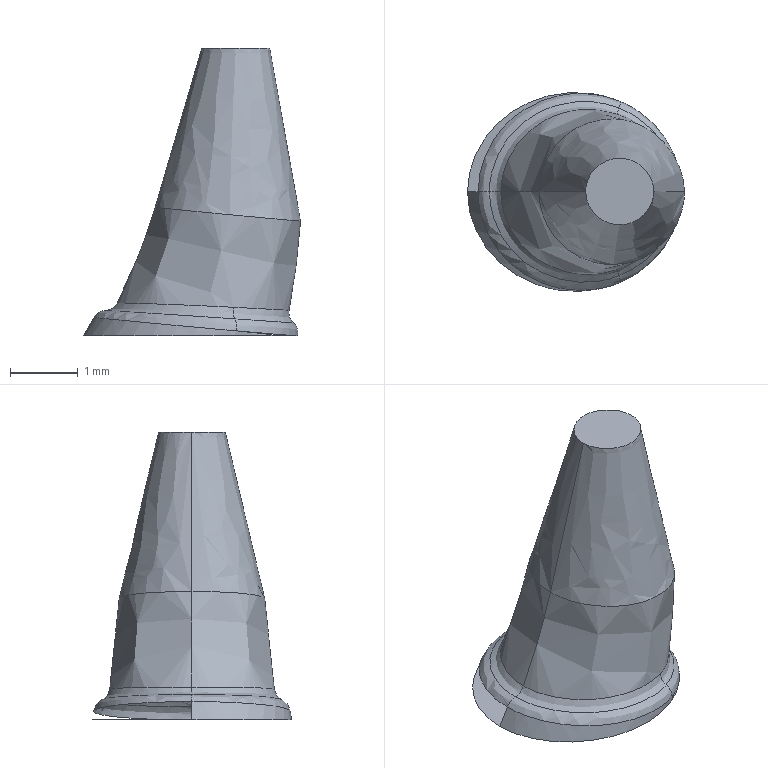Part | STEP file | solid 212 | 1 solid | 16 faces | box 3.206 x 2.939 x 4.252 mm | volume 13.592 mm3 | spline 14 | plane 2